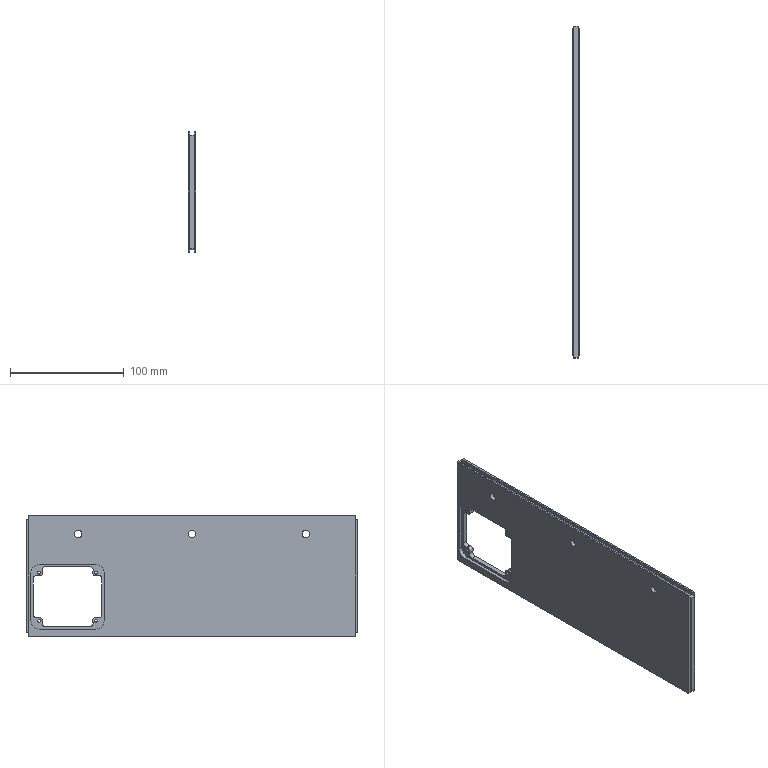Part | SolidWorks | features BaseBody 1 | 1 solid | 77 faces | box 7 x 292 x 106 mm | volume 184359 mm3 | cylinder 36 | plane 35 | cone 6 | commonest cylinder face diameters 6 x16 2.6 x8 6.4 x6 14.4 x4 19.617 x2